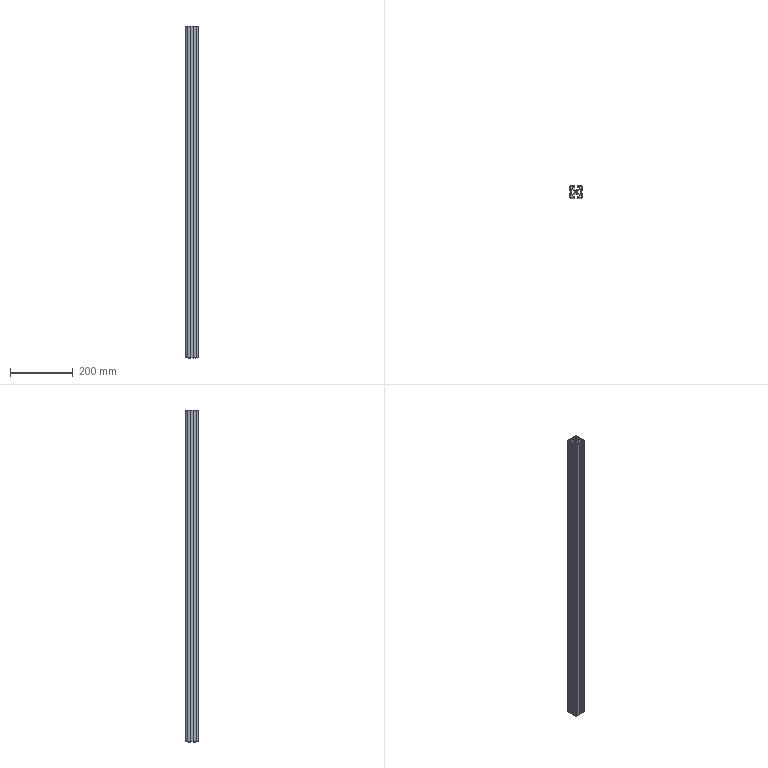Part | STEP file | LE-8-4040-S-OO_LE0314180216 | 1 solid | 188 faces | box 40 x 40 x 1060 mm | volume 506943 mm3 | cylinder 94 | plane 94 | commonest cylinder face diameters 0.6 x30 2 x28 4 x16 0.4 x8 6 x4 9 x4